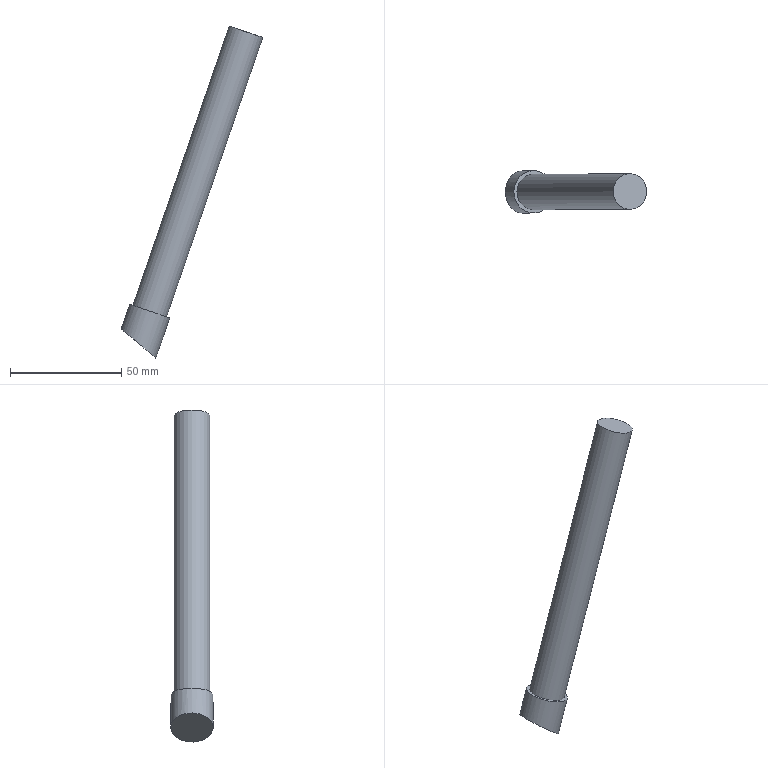Part | STEP file | solid 115 | 1 solid | 5 faces | box 63.638 x 19 x 149.358 mm | volume 31086 mm3 | plane 3 | cylinder 2 | commonest cylinder face diameters 16 x1 19 x1